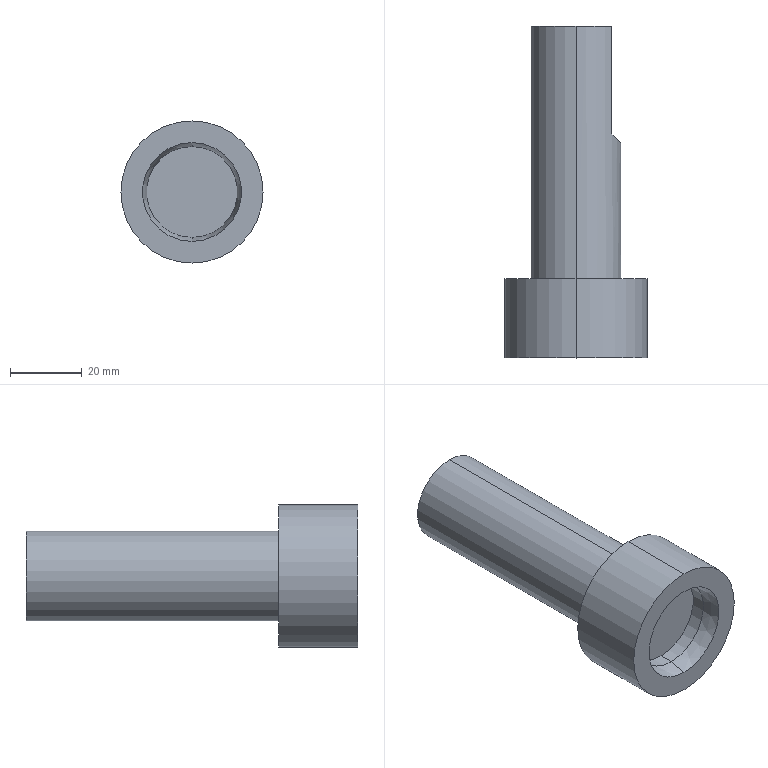Part | SolidWorks | features BaseBody 1 | 1 solid | 14 faces | box 39.5 x 92.2 x 39.5 mm | volume 55877 mm3 | cylinder 6 | plane 6 | cone 2 | commonest cylinder face diameters 25 x2 25.3 x2 39.5 x2
STEP:
#1=CARTESIAN_POINT('',(0.,-59.2,12.65));
#2=VERTEX_POINT('',#1);
#3=CARTESIAN_POINT('',(0.,-59.2,-12.65));
#4=VERTEX_POINT('',#3);
#5=CARTESIAN_POINT('',(0.,-59.2,0.));
#6=DIRECTION('',(0.,-1.,0.));
#7=DIRECTION('',(0.,0.,-1.));
#8=AXIS2_PLACEMENT_3D('',#5,#6,#7);
#9=CIRCLE('',#8,12.65);
#10=EDGE_CURVE('',#2,#4,#9,.T.);
#11=ORIENTED_EDGE('',*,*,#10,.F.);
#12=CARTESIAN_POINT('',(0.,-64.2,13.75));
#13=VERTEX_POINT('',#12);
#14=CARTESIAN_POINT('',(0.,-59.2,12.65));
#15=DIRECTION('',(0.,-0.9766,0.2149));
#16=VECTOR('',#15,1000.);
#17=LINE('',#14,#16);
#18=EDGE_CURVE('',#2,#13,#17,.T.);
#19=ORIENTED_EDGE('',*,*,#18,.T.);
#20=CARTESIAN_POINT('',(0.,-64.2,-13.75));
#21=VERTEX_POINT('',#20);
#22=CARTESIAN_POINT('',(0.,-64.2,0.));
#23=DIRECTION('',(0.,-1.,0.));
#24=DIRECTION('',(0.,0.,-1.));
#25=AXIS2_PLACEMENT_3D('',#22,#23,#24);
#26=CIRCLE('',#25,13.75);
#27=EDGE_CURVE('',#13,#21,#26,.T.);
#28=ORIENTED_EDGE('',*,*,#27,.T.);
#29=CARTESIAN_POINT('',(0.,-59.2,-12.65));
#30=DIRECTION('',(0.,-0.9766,-0.2149));
#31=VECTOR('',#30,1000.);
#32=LINE('',#29,#31);
#33=EDGE_CURVE('',#4,#21,#32,.T.);
#34=ORIENTED_EDGE('',*,*,#33,.F.);
#35=EDGE_LOOP('',(#11,#19,#28,#34));
#36=FACE_OUTER_BOUND('',#35,.T.);
#37=CARTESIAN_POINT('',(0.,-59.2,0.));
#38=DIRECTION('',(0.,-1.,0.));
#39=DIRECTION('',(0.,0.,-1.));
#40=AXIS2_PLACEMENT_3D('',#37,#38,#39);
#41=CONICAL_SURFACE('',#40,12.65,0.2166);
#42=ADVANCED_FACE('',(#36),#41,.F.);
#43=CARTESIAN_POINT('',(0.,-55.2,12.65));
#44=VERTEX_POINT('',#43);
#45=CARTESIAN_POINT('',(0.,-55.2,-12.65));
#46=VERTEX_POINT('',#45);
#47=CARTESIAN_POINT('',(0.,-55.2,0.));
#48=DIRECTION('',(0.,-1.,0.));
#49=DIRECTION('',(0.,0.,-1.));
#50=AXIS2_PLACEMENT_3D('',#47,#48,#49);
#51=CIRCLE('',#50,12.65);
#52=EDGE_CURVE('',#44,#46,#51,.T.);
#53=ORIENTED_EDGE('',*,*,#52,.F.);
#54=CARTESIAN_POINT('',(0.,-64.2,12.65));
#55=DIRECTION('',(0.,-1.,0.));
#56=VECTOR('',#55,1000.);
#57=LINE('',#54,#56);
#58=EDGE_CURVE('',#44,#2,#57,.T.);
#59=ORIENTED_EDGE('',*,*,#58,.T.);
#60=ORIENTED_EDGE('',*,*,#10,.T.);
#61=CARTESIAN_POINT('',(0.,-64.2,-12.65));
#62=DIRECTION('',(0.,-1.,0.));
#63=VECTOR('',#62,1000.);
#64=LINE('',#61,#63);
#65=EDGE_CURVE('',#46,#4,#64,.T.);
#66=ORIENTED_EDGE('',*,*,#65,.F.);
#67=EDGE_LOOP('',(#53,#59,#60,#66));
#68=FACE_OUTER_BOUND('',#67,.T.);
#69=CARTESIAN_POINT('',(0.,-64.2,0.));
#70=DIRECTION('',(0.,-1.,0.));
#71=DIRECTION('',(0.,0.,-1.));
#72=AXIS2_PLACEMENT_3D('',#69,#70,#71);
#73=CYLINDRICAL_SURFACE('',#72,12.65);
#74=ADVANCED_FACE('',(#68),#73,.F.);
#75=CARTESIAN_POINT('',(0.,-42.2,-19.75));
#76=VERTEX_POINT('',#75);
#77=CARTESIAN_POINT('',(0.,-42.2,19.75));
#78=VERTEX_POINT('',#77);
#79=CARTESIAN_POINT('',(0.,-42.2,0.));
#80=DIRECTION('',(0.,-1.,0.));
#81=DIRECTION('',(0.,0.,-1.));
#82=AXIS2_PLACEMENT_3D('',#79,#80,#81);
#83=CIRCLE('',#82,19.75);
#84=EDGE_CURVE('',#76,#78,#83,.T.);
#85=ORIENTED_EDGE('',*,*,#84,.T.);
#86=CARTESIAN_POINT('',(0.,-64.2,19.75));
#87=VERTEX_POINT('',#86);
#88=CARTESIAN_POINT('',(0.,-64.2,19.75));
#89=DIRECTION('',(0.,-1.,0.));
#90=VECTOR('',#89,1000.);
#91=LINE('',#88,#90);
#92=EDGE_CURVE('',#78,#87,#91,.T.);
#93=ORIENTED_EDGE('',*,*,#92,.T.);
#94=CARTESIAN_POINT('',(0.,-64.2,-19.75));
#95=VERTEX_POINT('',#94);
#96=CARTESIAN_POINT('',(0.,-64.2,0.));
#97=DIRECTION('',(0.,-1.,0.));
#98=DIRECTION('',(0.,0.,-1.));
#99=AXIS2_PLACEMENT_3D('',#96,#97,#98);
#100=CIRCLE('',#99,19.75);
#101=EDGE_CURVE('',#95,#87,#100,.T.);
#102=ORIENTED_EDGE('',*,*,#101,.F.);
#103=CARTESIAN_POINT('',(0.,-64.2,-19.75));
#104=DIRECTION('',(0.,-1.,0.));
#105=VECTOR('',#104,1000.);
#106=LINE('',#103,#105);
#107=EDGE_CURVE('',#76,#95,#106,.T.);
#108=ORIENTED_EDGE('',*,*,#107,.F.);
#109=EDGE_LOOP('',(#85,#93,#102,#108));
#110=FACE_OUTER_BOUND('',#109,.T.);
#111=CARTESIAN_POINT('',(0.,-64.2,0.));
#112=DIRECTION('',(0.,-1.,0.));
#113=DIRECTION('',(0.,0.,-1.));
#114=AXIS2_PLACEMENT_3D('',#111,#112,#113);
#115=CYLINDRICAL_SURFACE('',#114,19.75);
#116=ADVANCED_FACE('',(#110),#115,.T.);
#117=CARTESIAN_POINT('',(10.,28.,7.5));
#118=VERTEX_POINT('',#117);
#119=CARTESIAN_POINT('',(0.,28.,12.5));
#120=VERTEX_POINT('',#119);
#121=CARTESIAN_POINT('',(0.,28.,0.));
#122=DIRECTION('',(0.,-1.,0.));
#123=DIRECTION('',(0.,0.,-1.));
#124=AXIS2_PLACEMENT_3D('',#121,#122,#123);
#125=CIRCLE('',#124,12.5);
#126=EDGE_CURVE('',#118,#120,#125,.T.);
#127=ORIENTED_EDGE('',*,*,#126,.T.);
#128=CARTESIAN_POINT('',(0.,-42.2,12.5));
#129=VERTEX_POINT('',#128);
#130=CARTESIAN_POINT('',(0.,-64.2,12.5));
#131=DIRECTION('',(0.,-1.,0.));
#132=VECTOR('',#131,1000.);
#133=LINE('',#130,#132);
#134=EDGE_CURVE('',#120,#129,#133,.T.);
#135=ORIENTED_EDGE('',*,*,#134,.T.);
#136=CARTESIAN_POINT('',(0.,-42.2,-12.5));
#137=VERTEX_POINT('',#136);
#138=CARTESIAN_POINT('',(0.,-42.2,0.));
#139=DIRECTION('',(0.,-1.,0.));
#140=DIRECTION('',(0.,0.,-1.));
#141=AXIS2_PLACEMENT_3D('',#138,#139,#140);
#142=CIRCLE('',#141,12.5);
#143=EDGE_CURVE('',#137,#129,#142,.T.);
#144=ORIENTED_EDGE('',*,*,#143,.F.);
#145=CARTESIAN_POINT('',(0.,28.,-12.5));
#146=VERTEX_POINT('',#145);
#147=CARTESIAN_POINT('',(0.,-64.2,-12.5));
#148=DIRECTION('',(0.,-1.,0.));
#149=VECTOR('',#148,1000.);
#150=LINE('',#147,#149);
#151=EDGE_CURVE('',#146,#137,#150,.T.);
#152=ORIENTED_EDGE('',*,*,#151,.F.);
#153=CARTESIAN_POINT('',(10.,28.,-7.5));
#154=VERTEX_POINT('',#153);
#155=CARTESIAN_POINT('',(0.,28.,0.));
#156=DIRECTION('',(0.,-1.,0.));
#157=DIRECTION('',(0.,0.,-1.));
#158=AXIS2_PLACEMENT_3D('',#155,#156,#157);
#159=CIRCLE('',#158,12.5);
#160=EDGE_CURVE('',#146,#154,#159,.T.);
#161=ORIENTED_EDGE('',*,*,#160,.T.);
#162=CARTESIAN_POINT('',(10.,-2.,-7.5));
#163=VERTEX_POINT('',#162);
#164=CARTESIAN_POINT('',(10.,-64.2,-7.5));
#165=DIRECTION('',(0.,1.,0.));
#166=VECTOR('',#165,1000.);
#167=LINE('',#164,#166);
#168=EDGE_CURVE('',#163,#154,#167,.T.);
#169=ORIENTED_EDGE('',*,*,#168,.F.);
#170=CARTESIAN_POINT('',(10.,-2.,7.5));
#171=VERTEX_POINT('',#170);
#172=CARTESIAN_POINT('',(10.,-2.,7.5));
#173=CARTESIAN_POINT('',(13.462,-5.462,2.885));
#174=CARTESIAN_POINT('',(13.462,-5.462,-2.885));
#175=CARTESIAN_POINT('',(10.,-2.,-7.5));
#176=(BOUNDED_CURVE()B_SPLINE_CURVE(3,(#172,#173,#174,#175),.UNSPECIFIED.,.F.,.F.)B_SPLINE_CURVE_WITH_KNOTS((4,4),(5.64,6.927),.UNSPECIFIED.)CURVE()GEOMETRIC_REPRESENTATION_ITEM()RATIONAL_B_SPLINE_CURVE((1.,0.8667,0.8667,1.))REPRESENTATION_ITEM(''));
#177=EDGE_CURVE('',#171,#163,#176,.T.);
#178=ORIENTED_EDGE('',*,*,#177,.F.);
#179=CARTESIAN_POINT('',(10.,-64.2,7.5));
#180=DIRECTION('',(0.,-1.,0.));
#181=VECTOR('',#180,1000.);
#182=LINE('',#179,#181);
#183=EDGE_CURVE('',#118,#171,#182,.T.);
#184=ORIENTED_EDGE('',*,*,#183,.F.);
#185=EDGE_LOOP('',(#127,#135,#144,#152,#161,#169,#178,#184));
#186=FACE_OUTER_BOUND('',#185,.T.);
#187=CARTESIAN_POINT('',(0.,-64.2,0.));
#188=DIRECTION('',(0.,-1.,0.));
#189=DIRECTION('',(0.,0.,-1.));
#190=AXIS2_PLACEMENT_3D('',#187,#188,#189);
#191=CYLINDRICAL_SURFACE('',#190,12.5);
#192=ADVANCED_FACE('',(#186),#191,.T.);
#193=CARTESIAN_POINT('',(10.,-2.,12.5));
#194=DIRECTION('',(0.,0.,-1.));
#195=VECTOR('',#194,1000.);
#196=LINE('',#193,#195);
#197=EDGE_CURVE('',#171,#163,#196,.T.);
#198=ORIENTED_EDGE('',*,*,#197,.F.);
#199=ORIENTED_EDGE('',*,*,#177,.T.);
#200=EDGE_LOOP('',(#198,#199));
#201=FACE_OUTER_BOUND('',#200,.T.);
#202=CARTESIAN_POINT('',(10.,-2.,12.5));
#203=DIRECTION('',(0.7071,0.7071,0.));
#204=DIRECTION('',(0.,0.,-1.));
#205=AXIS2_PLACEMENT_3D('',#202,#203,#204);
#206=PLANE('',#205);
#207=ADVANCED_FACE('',(#201),#206,.T.);
#208=ORIENTED_EDGE('',*,*,#183,.T.);
#209=ORIENTED_EDGE('',*,*,#197,.T.);
#210=ORIENTED_EDGE('',*,*,#168,.T.);
#211=CARTESIAN_POINT('',(10.,28.,12.5));
#212=DIRECTION('',(0.,0.,-1.));
#213=VECTOR('',#212,1000.);
#214=LINE('',#211,#213);
#215=EDGE_CURVE('',#118,#154,#214,.T.);
#216=ORIENTED_EDGE('',*,*,#215,.F.);
#217=EDGE_LOOP('',(#208,#209,#210,#216));
#218=FACE_OUTER_BOUND('',#217,.T.);
#219=CARTESIAN_POINT('',(10.,28.,12.5));
#220=DIRECTION('',(1.,0.,0.));
#221=DIRECTION('',(0.,1.,0.));
#222=AXIS2_PLACEMENT_3D('',#219,#220,#221);
#223=PLANE('',#222);
#224=ADVANCED_FACE('',(#218),#223,.T.);
#225=CARTESIAN_POINT('',(0.,-55.2,0.));
#226=DIRECTION('',(0.,-1.,0.));
#227=DIRECTION('',(0.,0.,-1.));
#228=AXIS2_PLACEMENT_3D('',#225,#226,#227);
#229=CIRCLE('',#228,12.65);
#230=EDGE_CURVE('',#46,#44,#229,.T.);
#231=ORIENTED_EDGE('',*,*,#230,.T.);
#232=ORIENTED_EDGE('',*,*,#52,.T.);
#233=EDGE_LOOP('',(#231,#232));
#234=FACE_OUTER_BOUND('',#233,.T.);
#235=CARTESIAN_POINT('',(0.,-55.2,0.));
#236=DIRECTION('',(0.,-1.,0.));
#237=DIRECTION('',(0.,0.,-1.));
#238=AXIS2_PLACEMENT_3D('',#235,#236,#237);
#239=PLANE('',#238);
#240=ADVANCED_FACE('',(#234),#239,.T.);
#241=CARTESIAN_POINT('',(0.,-64.2,0.));
#242=DIRECTION('',(0.,-1.,0.));
#243=DIRECTION('',(0.,0.,-1.));
#244=AXIS2_PLACEMENT_3D('',#241,#242,#243);
#245=CIRCLE('',#244,13.75);
#246=EDGE_CURVE('',#21,#13,#245,.T.);
#247=ORIENTED_EDGE('',*,*,#246,.F.);
#248=ORIENTED_EDGE('',*,*,#27,.F.);
#249=EDGE_LOOP('',(#247,#248));
#250=FACE_BOUND('',#249,.T.);
#251=ORIENTED_EDGE('',*,*,#101,.T.);
#252=CARTESIAN_POINT('',(0.,-64.2,0.));
#253=DIRECTION('',(0.,-1.,0.));
#254=DIRECTION('',(0.,0.,-1.));
#255=AXIS2_PLACEMENT_3D('',#252,#253,#254);
#256=CIRCLE('',#255,19.75);
#257=EDGE_CURVE('',#87,#95,#256,.T.);
#258=ORIENTED_EDGE('',*,*,#257,.T.);
#259=EDGE_LOOP('',(#251,#258));
#260=FACE_OUTER_BOUND('',#259,.T.);
#261=CARTESIAN_POINT('',(19.75,-64.2,0.));
#262=DIRECTION('',(0.,1.,0.));
#263=DIRECTION('',(1.,0.,0.));
#264=AXIS2_PLACEMENT_3D('',#261,#262,#263);
#265=PLANE('',#264);
#266=ADVANCED_FACE('',(#250,#260),#265,.F.);
#267=ORIENTED_EDGE('',*,*,#143,.T.);
#268=CARTESIAN_POINT('',(0.,-42.2,0.));
#269=DIRECTION('',(0.,-1.,0.));
#270=DIRECTION('',(0.,0.,-1.));
#271=AXIS2_PLACEMENT_3D('',#268,#269,#270);
#272=CIRCLE('',#271,12.5);
#273=EDGE_CURVE('',#129,#137,#272,.T.);
#274=ORIENTED_EDGE('',*,*,#273,.T.);
#275=EDGE_LOOP('',(#267,#274));
#276=FACE_BOUND('',#275,.T.);
#277=ORIENTED_EDGE('',*,*,#84,.F.);
#278=CARTESIAN_POINT('',(0.,-42.2,0.));
#279=DIRECTION('',(0.,-1.,0.));
#280=DIRECTION('',(0.,0.,-1.));
#281=AXIS2_PLACEMENT_3D('',#278,#279,#280);
#282=CIRCLE('',#281,19.75);
#283=EDGE_CURVE('',#78,#76,#282,.T.);
#284=ORIENTED_EDGE('',*,*,#283,.F.);
#285=EDGE_LOOP('',(#277,#284));
#286=FACE_OUTER_BOUND('',#285,.T.);
#287=CARTESIAN_POINT('',(12.5,-42.2,0.));
#288=DIRECTION('',(0.,-1.,0.));
#289=DIRECTION('',(0.,0.,-1.));
#290=AXIS2_PLACEMENT_3D('',#287,#288,#289);
#291=PLANE('',#290);
#292=ADVANCED_FACE('',(#276,#286),#291,.F.);
#293=ORIENTED_EDGE('',*,*,#215,.T.);
#294=ORIENTED_EDGE('',*,*,#160,.F.);
#295=CARTESIAN_POINT('',(0.,28.,0.));
#296=DIRECTION('',(0.,-1.,0.));
#297=DIRECTION('',(0.,0.,-1.));
#298=AXIS2_PLACEMENT_3D('',#295,#296,#297);
#299=CIRCLE('',#298,12.5);
#300=EDGE_CURVE('',#120,#146,#299,.T.);
#301=ORIENTED_EDGE('',*,*,#300,.F.);
#302=ORIENTED_EDGE('',*,*,#126,.F.);
#303=EDGE_LOOP('',(#293,#294,#301,#302));
#304=FACE_OUTER_BOUND('',#303,.T.);
#305=CARTESIAN_POINT('',(0.,28.,0.));
#306=DIRECTION('',(0.,-1.,0.));
#307=DIRECTION('',(0.,0.,-1.));
#308=AXIS2_PLACEMENT_3D('',#305,#306,#307);
#309=PLANE('',#308);
#310=ADVANCED_FACE('',(#304),#309,.F.);
#311=ORIENTED_EDGE('',*,*,#134,.F.);
#312=ORIENTED_EDGE('',*,*,#300,.T.);
#313=ORIENTED_EDGE('',*,*,#151,.T.);
#314=ORIENTED_EDGE('',*,*,#273,.F.);
#315=EDGE_LOOP('',(#311,#312,#313,#314));
#316=FACE_OUTER_BOUND('',#315,.T.);
#317=CARTESIAN_POINT('',(0.,-64.2,0.));
#318=DIRECTION('',(0.,-1.,0.));
#319=DIRECTION('',(0.,0.,-1.));
#320=AXIS2_PLACEMENT_3D('',#317,#318,#319);
#321=CYLINDRICAL_SURFACE('',#320,12.5);
#322=ADVANCED_FACE('',(#316),#321,.T.);
#323=ORIENTED_EDGE('',*,*,#92,.F.);
#324=ORIENTED_EDGE('',*,*,#283,.T.);
#325=ORIENTED_EDGE('',*,*,#107,.T.);
#326=ORIENTED_EDGE('',*,*,#257,.F.);
#327=EDGE_LOOP('',(#323,#324,#325,#326));
#328=FACE_OUTER_BOUND('',#327,.T.);
#329=CARTESIAN_POINT('',(0.,-64.2,0.));
#330=DIRECTION('',(0.,-1.,0.));
#331=DIRECTION('',(0.,0.,-1.));
#332=AXIS2_PLACEMENT_3D('',#329,#330,#331);
#333=CYLINDRICAL_SURFACE('',#332,19.75);
#334=ADVANCED_FACE('',(#328),#333,.T.);
#335=ORIENTED_EDGE('',*,*,#58,.F.);
#336=ORIENTED_EDGE('',*,*,#230,.F.);
#337=ORIENTED_EDGE('',*,*,#65,.T.);
#338=CARTESIAN_POINT('',(0.,-59.2,0.));
#339=DIRECTION('',(0.,-1.,0.));
#340=DIRECTION('',(0.,0.,-1.));
#341=AXIS2_PLACEMENT_3D('',#338,#339,#340);
#342=CIRCLE('',#341,12.65);
#343=EDGE_CURVE('',#4,#2,#342,.T.);
#344=ORIENTED_EDGE('',*,*,#343,.T.);
#345=EDGE_LOOP('',(#335,#336,#337,#344));
#346=FACE_OUTER_BOUND('',#345,.T.);
#347=CARTESIAN_POINT('',(0.,-64.2,0.));
#348=DIRECTION('',(0.,-1.,0.));
#349=DIRECTION('',(0.,0.,-1.));
#350=AXIS2_PLACEMENT_3D('',#347,#348,#349);
#351=CYLINDRICAL_SURFACE('',#350,12.65);
#352=ADVANCED_FACE('',(#346),#351,.F.);
#353=ORIENTED_EDGE('',*,*,#18,.F.);
#354=ORIENTED_EDGE('',*,*,#343,.F.);
#355=ORIENTED_EDGE('',*,*,#33,.T.);
#356=ORIENTED_EDGE('',*,*,#246,.T.);
#357=EDGE_LOOP('',(#353,#354,#355,#356));
#358=FACE_OUTER_BOUND('',#357,.T.);
#359=CARTESIAN_POINT('',(0.,-59.2,0.));
#360=DIRECTION('',(0.,-1.,0.));
#361=DIRECTION('',(0.,0.,-1.));
#362=AXIS2_PLACEMENT_3D('',#359,#360,#361);
#363=CONICAL_SURFACE('',#362,12.65,0.2166);
#364=ADVANCED_FACE('',(#358),#363,.F.);
#365=CLOSED_SHELL('',(#42,#74,#116,#192,#207,#224,#240,#266,#292,#310,#322,#334,#352,#364));
#366=MANIFOLD_SOLID_BREP('',#365);
#367=CARTESIAN_POINT('',(0.,0.,0.));
#368=DIRECTION('',(0.,0.,1.));
#369=DIRECTION('',(1.,0.,0.));
#370=AXIS2_PLACEMENT_3D('',#367,#368,#369);
#371=(LENGTH_UNIT()NAMED_UNIT(*)SI_UNIT(.MILLI.,.METRE.));
#372=UNCERTAINTY_MEASURE_WITH_UNIT(LENGTH_MEASURE(0.00001),#371,'','');
#373=(NAMED_UNIT(*)PLANE_ANGLE_UNIT()SI_UNIT($,.RADIAN.));
#374=(NAMED_UNIT(*)SI_UNIT($,.STERADIAN.)SOLID_ANGLE_UNIT());
#375=(GEOMETRIC_REPRESENTATION_CONTEXT(3)GLOBAL_UNCERTAINTY_ASSIGNED_CONTEXT((#372))GLOBAL_UNIT_ASSIGNED_CONTEXT((#371,#373,#374))REPRESENTATION_CONTEXT('',''));
#376=ADVANCED_BREP_SHAPE_REPRESENTATION('',(#366,#370),#375);